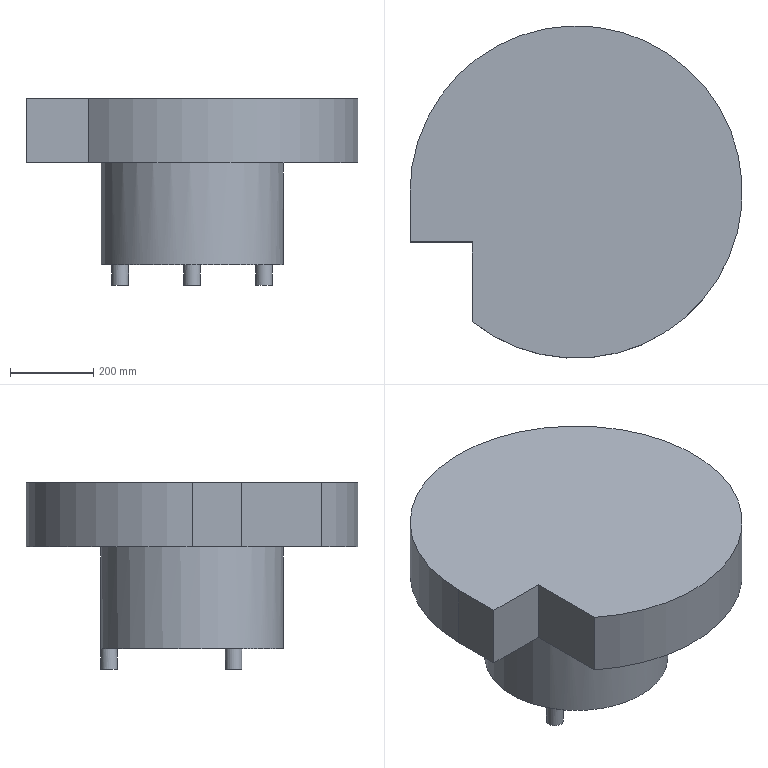Part | STEP file | ALIMENTADOR_ARRUELA | 1 solid | 14 faces | box 800 x 800 x 450 mm | volume 113086598 mm3 | plane 9 | cylinder 5 | commonest cylinder face diameters 40 x3 440 x1 800 x1
STEP:
#1=CARTESIAN_POINT('',(0.,0.,0.));
#2=DIRECTION('',(0.,0.,1.));
#3=DIRECTION('',(1.,0.,0.));
#4=AXIS2_PLACEMENT_3D('',#1,#2,#3);
#5=CARTESIAN_POINT('',(0.,220.,0.));
#6=VERTEX_POINT('',#5);
#7=CARTESIAN_POINT('',(-20.,200.,0.));
#8=VERTEX_POINT('',#7);
#9=CARTESIAN_POINT('',(0.,200.,0.));
#10=DIRECTION('',(0.,0.,-1.));
#11=DIRECTION('',(1.,0.,0.));
#12=AXIS2_PLACEMENT_3D('',#9,#10,#11);
#13=CIRCLE('',#12,20.);
#14=CARTESIAN_POINT('',(0.,200.,25.));
#15=DIRECTION('',(0.,0.,-1.));
#16=DIRECTION('',(1.,0.,0.));
#17=AXIS2_PLACEMENT_3D('',#14,#15,#16);
#18=CYLINDRICAL_SURFACE('',#17,20.);
#19=CARTESIAN_POINT('',(0.,25.));
#20=DIRECTION('',(1.,0.));
#21=VECTOR('',#20,1.);
#22=LINE('',#19,#21);
#23=(GEOMETRIC_REPRESENTATION_CONTEXT(2)PARAMETRIC_REPRESENTATION_CONTEXT()REPRESENTATION_CONTEXT('',''));
#24=DEFINITIONAL_REPRESENTATION('',(#22),#23);
#25=PCURVE('',#18,#24);
#26=CARTESIAN_POINT('',(0.,0.,0.));
#27=DIRECTION('',(0.,0.,-1.));
#28=DIRECTION('',(-1.,0.,0.));
#29=AXIS2_PLACEMENT_3D('',#26,#27,#28);
#30=PLANE('',#29);
#31=CARTESIAN_POINT('',(0.,200.));
#32=DIRECTION('',(-1.,0.));
#33=AXIS2_PLACEMENT_2D('',#31,#32);
#34=CIRCLE('',#33,20.);
#35=(GEOMETRIC_REPRESENTATION_CONTEXT(2)PARAMETRIC_REPRESENTATION_CONTEXT()REPRESENTATION_CONTEXT('',''));
#36=DEFINITIONAL_REPRESENTATION('',(#34),#35);
#37=PCURVE('',#30,#36);
#38=SURFACE_CURVE('',#13,(#25,#37),.PCURVE_S1.);
#39=EDGE_CURVE('',#6,#8,#38,.T.);
#40=ORIENTED_EDGE('',*,*,#39,.F.);
#41=CARTESIAN_POINT('',(0.,220.,50.));
#42=VERTEX_POINT('',#41);
#43=CARTESIAN_POINT('',(0.,220.,50.));
#44=CARTESIAN_POINT('',(0.,220.,0.));
#45=B_SPLINE_CURVE_WITH_KNOTS('',1,(#43,#44),.UNSPECIFIED.,.F.,.F.,(2,2),(-25.,25.),.PIECEWISE_BEZIER_KNOTS.);
#46=CARTESIAN_POINT('',(4.712,0.));
#47=DIRECTION('',(0.,1.));
#48=VECTOR('',#47,1.);
#49=LINE('',#46,#48);
#50=(GEOMETRIC_REPRESENTATION_CONTEXT(2)PARAMETRIC_REPRESENTATION_CONTEXT()REPRESENTATION_CONTEXT('',''));
#51=DEFINITIONAL_REPRESENTATION('',(#49),#50);
#52=PCURVE('',#18,#51);
#53=CARTESIAN_POINT('',(10.996,0.));
#54=DIRECTION('',(0.,1.));
#55=VECTOR('',#54,1.);
#56=LINE('',#53,#55);
#57=(GEOMETRIC_REPRESENTATION_CONTEXT(2)PARAMETRIC_REPRESENTATION_CONTEXT()REPRESENTATION_CONTEXT('',''));
#58=DEFINITIONAL_REPRESENTATION('',(#56),#57);
#59=PCURVE('',#18,#58);
#60=SEAM_CURVE('',#45,(#52,#59),.PCURVE_S1.);
#61=EDGE_CURVE('',#42,#6,#60,.T.);
#62=ORIENTED_EDGE('',*,*,#61,.F.);
#63=CARTESIAN_POINT('',(0.,220.,50.));
#64=VERTEX_POINT('',#63);
#65=CARTESIAN_POINT('',(0.,200.,50.));
#66=DIRECTION('',(0.,0.,-1.));
#67=DIRECTION('',(1.,0.,0.));
#68=AXIS2_PLACEMENT_3D('',#65,#66,#67);
#69=CIRCLE('',#68,20.);
#70=CARTESIAN_POINT('',(0.,-25.));
#71=DIRECTION('',(1.,0.));
#72=VECTOR('',#71,1.);
#73=LINE('',#70,#72);
#74=(GEOMETRIC_REPRESENTATION_CONTEXT(2)PARAMETRIC_REPRESENTATION_CONTEXT()REPRESENTATION_CONTEXT('',''));
#75=DEFINITIONAL_REPRESENTATION('',(#73),#74);
#76=PCURVE('',#18,#75);
#77=CARTESIAN_POINT('',(-220.,0.,50.));
#78=DIRECTION('',(0.,0.,1.));
#79=DIRECTION('',(1.,0.,0.));
#80=AXIS2_PLACEMENT_3D('',#77,#78,#79);
#81=PLANE('',#80);
#82=CARTESIAN_POINT('',(240.,200.));
#83=CARTESIAN_POINT('',(240.,165.359));
#84=CARTESIAN_POINT('',(210.,182.679));
#85=CARTESIAN_POINT('',(180.,200.));
#86=CARTESIAN_POINT('',(210.,217.321));
#87=CARTESIAN_POINT('',(240.,234.641));
#88=CARTESIAN_POINT('',(240.,200.));
#89=(BOUNDED_CURVE()B_SPLINE_CURVE(2,(#82,#83,#84,#85,#86,#87,#88),.UNSPECIFIED.,.T.,.F.)B_SPLINE_CURVE_WITH_KNOTS((1,2,2,2,2,1),(-2.094,0.,2.094,4.189,6.283,8.378),.UNSPECIFIED.)CURVE()GEOMETRIC_REPRESENTATION_ITEM()RATIONAL_B_SPLINE_CURVE((1.,0.5,1.,0.5,1.,0.5,1.))REPRESENTATION_ITEM(''));
#90=(GEOMETRIC_REPRESENTATION_CONTEXT(2)PARAMETRIC_REPRESENTATION_CONTEXT()REPRESENTATION_CONTEXT('',''));
#91=DEFINITIONAL_REPRESENTATION('',(#89),#90);
#92=PCURVE('',#81,#91);
#93=SURFACE_CURVE('',#69,(#76,#92),.PCURVE_S1.);
#94=EDGE_CURVE('',#64,#42,#93,.T.);
#95=ORIENTED_EDGE('',*,*,#94,.T.);
#96=ORIENTED_EDGE('',*,*,#61,.T.);
#97=CARTESIAN_POINT('',(0.,200.,0.));
#98=DIRECTION('',(0.,0.,-1.));
#99=DIRECTION('',(1.,0.,0.));
#100=AXIS2_PLACEMENT_3D('',#97,#98,#99);
#101=CIRCLE('',#100,20.);
#102=CARTESIAN_POINT('',(6.283,25.));
#103=DIRECTION('',(1.,0.));
#104=VECTOR('',#103,1.);
#105=LINE('',#102,#104);
#106=(GEOMETRIC_REPRESENTATION_CONTEXT(2)PARAMETRIC_REPRESENTATION_CONTEXT()REPRESENTATION_CONTEXT('',''));
#107=DEFINITIONAL_REPRESENTATION('',(#105),#106);
#108=PCURVE('',#18,#107);
#109=CARTESIAN_POINT('',(0.,200.));
#110=DIRECTION('',(-1.,0.));
#111=AXIS2_PLACEMENT_2D('',#109,#110);
#112=CIRCLE('',#111,20.);
#113=(GEOMETRIC_REPRESENTATION_CONTEXT(2)PARAMETRIC_REPRESENTATION_CONTEXT()REPRESENTATION_CONTEXT('',''));
#114=DEFINITIONAL_REPRESENTATION('',(#112),#113);
#115=PCURVE('',#30,#114);
#116=SURFACE_CURVE('',#101,(#108,#115),.PCURVE_S1.);
#117=EDGE_CURVE('',#8,#6,#116,.T.);
#118=ORIENTED_EDGE('',*,*,#117,.F.);
#119=EDGE_LOOP('',(#40,#62,#95,#96,#118));
#120=FACE_BOUND('',#119,.T.);
#121=ADVANCED_FACE('',(#120),#18,.T.);
#122=CARTESIAN_POINT('',(-190.526,-110.,50.));
#123=VERTEX_POINT('',#122);
#124=CARTESIAN_POINT('',(190.526,-110.,50.));
#125=VERTEX_POINT('',#124);
#126=CARTESIAN_POINT('',(0.,0.,50.));
#127=DIRECTION('',(0.,0.,1.));
#128=DIRECTION('',(1.,0.,0.));
#129=AXIS2_PLACEMENT_3D('',#126,#127,#128);
#130=CIRCLE('',#129,220.);
#131=CARTESIAN_POINT('',(220.,0.));
#132=DIRECTION('',(1.,0.));
#133=AXIS2_PLACEMENT_2D('',#131,#132);
#134=CIRCLE('',#133,220.);
#135=(GEOMETRIC_REPRESENTATION_CONTEXT(2)PARAMETRIC_REPRESENTATION_CONTEXT()REPRESENTATION_CONTEXT('',''));
#136=DEFINITIONAL_REPRESENTATION('',(#134),#135);
#137=PCURVE('',#81,#136);
#138=CARTESIAN_POINT('',(0.,0.,250.));
#139=DIRECTION('',(0.,0.,1.));
#140=DIRECTION('',(-0.8776,-0.4794,0.));
#141=AXIS2_PLACEMENT_3D('',#138,#139,#140);
#142=CYLINDRICAL_SURFACE('',#141,220.);
#143=CARTESIAN_POINT('',(-3.642,-200.));
#144=DIRECTION('',(1.,0.));
#145=VECTOR('',#144,1.);
#146=LINE('',#143,#145);
#147=(GEOMETRIC_REPRESENTATION_CONTEXT(2)PARAMETRIC_REPRESENTATION_CONTEXT()REPRESENTATION_CONTEXT('',''));
#148=DEFINITIONAL_REPRESENTATION('',(#146),#147);
#149=PCURVE('',#142,#148);
#150=SURFACE_CURVE('',#130,(#137,#149),.PCURVE_S1.);
#151=EDGE_CURVE('',#123,#125,#150,.T.);
#152=ORIENTED_EDGE('',*,*,#151,.T.);
#153=CARTESIAN_POINT('',(0.,0.,50.));
#154=DIRECTION('',(0.,0.,1.));
#155=DIRECTION('',(1.,0.,0.));
#156=AXIS2_PLACEMENT_3D('',#153,#154,#155);
#157=CIRCLE('',#156,220.);
#158=CARTESIAN_POINT('',(220.,0.));
#159=DIRECTION('',(1.,0.));
#160=AXIS2_PLACEMENT_2D('',#158,#159);
#161=CIRCLE('',#160,220.);
#162=(GEOMETRIC_REPRESENTATION_CONTEXT(2)PARAMETRIC_REPRESENTATION_CONTEXT()REPRESENTATION_CONTEXT('',''));
#163=DEFINITIONAL_REPRESENTATION('',(#161),#162);
#164=PCURVE('',#81,#163);
#165=CARTESIAN_POINT('',(-3.642,-200.));
#166=DIRECTION('',(1.,0.));
#167=VECTOR('',#166,1.);
#168=LINE('',#165,#167);
#169=(GEOMETRIC_REPRESENTATION_CONTEXT(2)PARAMETRIC_REPRESENTATION_CONTEXT()REPRESENTATION_CONTEXT('',''));
#170=DEFINITIONAL_REPRESENTATION('',(#168),#169);
#171=PCURVE('',#142,#170);
#172=SURFACE_CURVE('',#157,(#164,#171),.PCURVE_S1.);
#173=EDGE_CURVE('',#125,#42,#172,.T.);
#174=ORIENTED_EDGE('',*,*,#173,.T.);
#175=CARTESIAN_POINT('',(-193.068,-105.474,50.));
#176=VERTEX_POINT('',#175);
#177=CARTESIAN_POINT('',(0.,0.,50.));
#178=DIRECTION('',(0.,0.,1.));
#179=DIRECTION('',(1.,0.,0.));
#180=AXIS2_PLACEMENT_3D('',#177,#178,#179);
#181=CIRCLE('',#180,220.);
#182=CARTESIAN_POINT('',(220.,0.));
#183=DIRECTION('',(1.,0.));
#184=AXIS2_PLACEMENT_2D('',#182,#183);
#185=CIRCLE('',#184,220.);
#186=(GEOMETRIC_REPRESENTATION_CONTEXT(2)PARAMETRIC_REPRESENTATION_CONTEXT()REPRESENTATION_CONTEXT('',''));
#187=DEFINITIONAL_REPRESENTATION('',(#185),#186);
#188=PCURVE('',#81,#187);
#189=CARTESIAN_POINT('',(2.642,-200.));
#190=DIRECTION('',(1.,0.));
#191=VECTOR('',#190,1.);
#192=LINE('',#189,#191);
#193=(GEOMETRIC_REPRESENTATION_CONTEXT(2)PARAMETRIC_REPRESENTATION_CONTEXT()REPRESENTATION_CONTEXT('',''));
#194=DEFINITIONAL_REPRESENTATION('',(#192),#193);
#195=PCURVE('',#142,#194);
#196=SURFACE_CURVE('',#181,(#188,#195),.PCURVE_S1.);
#197=EDGE_CURVE('',#42,#176,#196,.T.);
#198=ORIENTED_EDGE('',*,*,#197,.T.);
#199=CARTESIAN_POINT('',(0.,0.,50.));
#200=DIRECTION('',(0.,0.,1.));
#201=DIRECTION('',(1.,0.,0.));
#202=AXIS2_PLACEMENT_3D('',#199,#200,#201);
#203=CIRCLE('',#202,220.);
#204=CARTESIAN_POINT('',(220.,0.));
#205=DIRECTION('',(1.,0.));
#206=AXIS2_PLACEMENT_2D('',#204,#205);
#207=CIRCLE('',#206,220.);
#208=(GEOMETRIC_REPRESENTATION_CONTEXT(2)PARAMETRIC_REPRESENTATION_CONTEXT()REPRESENTATION_CONTEXT('',''));
#209=DEFINITIONAL_REPRESENTATION('',(#207),#208);
#210=PCURVE('',#81,#209);
#211=CARTESIAN_POINT('',(-3.642,-200.));
#212=DIRECTION('',(1.,0.));
#213=VECTOR('',#212,1.);
#214=LINE('',#211,#213);
#215=(GEOMETRIC_REPRESENTATION_CONTEXT(2)PARAMETRIC_REPRESENTATION_CONTEXT()REPRESENTATION_CONTEXT('',''));
#216=DEFINITIONAL_REPRESENTATION('',(#214),#215);
#217=PCURVE('',#142,#216);
#218=SURFACE_CURVE('',#203,(#210,#217),.PCURVE_S1.);
#219=EDGE_CURVE('',#176,#123,#218,.T.);
#220=ORIENTED_EDGE('',*,*,#219,.T.);
#221=EDGE_LOOP('',(#152,#174,#198,#220));
#222=FACE_BOUND('',#221,.F.);
#223=CARTESIAN_POINT('',(190.526,-110.,50.));
#224=VERTEX_POINT('',#223);
#225=CARTESIAN_POINT('',(173.205,-100.,50.));
#226=DIRECTION('',(0.,0.,1.));
#227=DIRECTION('',(1.,0.,0.));
#228=AXIS2_PLACEMENT_3D('',#225,#226,#227);
#229=CIRCLE('',#228,20.);
#230=CARTESIAN_POINT('',(393.205,-100.));
#231=DIRECTION('',(1.,0.));
#232=AXIS2_PLACEMENT_2D('',#230,#231);
#233=CIRCLE('',#232,20.);
#234=(GEOMETRIC_REPRESENTATION_CONTEXT(2)PARAMETRIC_REPRESENTATION_CONTEXT()REPRESENTATION_CONTEXT('',''));
#235=DEFINITIONAL_REPRESENTATION('',(#233),#234);
#236=PCURVE('',#81,#235);
#237=CARTESIAN_POINT('',(173.205,-100.,25.));
#238=DIRECTION('',(0.,0.,-1.));
#239=DIRECTION('',(-0.5,-0.866,0.));
#240=AXIS2_PLACEMENT_3D('',#237,#238,#239);
#241=CYLINDRICAL_SURFACE('',#240,20.);
#242=CARTESIAN_POINT('',(16.755,-25.));
#243=DIRECTION('',(-1.,0.));
#244=VECTOR('',#243,1.);
#245=LINE('',#242,#244);
#246=(GEOMETRIC_REPRESENTATION_CONTEXT(2)PARAMETRIC_REPRESENTATION_CONTEXT()REPRESENTATION_CONTEXT('',''));
#247=DEFINITIONAL_REPRESENTATION('',(#245),#246);
#248=PCURVE('',#241,#247);
#249=SURFACE_CURVE('',#229,(#236,#248),.PCURVE_S1.);
#250=EDGE_CURVE('',#125,#224,#249,.T.);
#251=ORIENTED_EDGE('',*,*,#250,.F.);
#252=EDGE_LOOP('',(#251));
#253=FACE_BOUND('',#252,.F.);
#254=ORIENTED_EDGE('',*,*,#94,.T.);
#255=EDGE_LOOP('',(#254));
#256=FACE_BOUND('',#255,.F.);
#257=CARTESIAN_POINT('',(-190.526,-110.,50.));
#258=VERTEX_POINT('',#257);
#259=CARTESIAN_POINT('',(-173.205,-100.,50.));
#260=DIRECTION('',(0.,0.,1.));
#261=DIRECTION('',(1.,0.,0.));
#262=AXIS2_PLACEMENT_3D('',#259,#260,#261);
#263=CIRCLE('',#262,20.);
#264=CARTESIAN_POINT('',(46.795,-100.));
#265=DIRECTION('',(1.,0.));
#266=AXIS2_PLACEMENT_2D('',#264,#265);
#267=CIRCLE('',#266,20.);
#268=(GEOMETRIC_REPRESENTATION_CONTEXT(2)PARAMETRIC_REPRESENTATION_CONTEXT()REPRESENTATION_CONTEXT('',''));
#269=DEFINITIONAL_REPRESENTATION('',(#267),#268);
#270=PCURVE('',#81,#269);
#271=CARTESIAN_POINT('',(-173.205,-100.,25.));
#272=DIRECTION('',(0.,0.,-1.));
#273=DIRECTION('',(-0.5,0.866,0.));
#274=AXIS2_PLACEMENT_3D('',#271,#272,#273);
#275=CYLINDRICAL_SURFACE('',#274,20.);
#276=CARTESIAN_POINT('',(14.661,-25.));
#277=DIRECTION('',(-1.,0.));
#278=VECTOR('',#277,1.);
#279=LINE('',#276,#278);
#280=(GEOMETRIC_REPRESENTATION_CONTEXT(2)PARAMETRIC_REPRESENTATION_CONTEXT()REPRESENTATION_CONTEXT('',''));
#281=DEFINITIONAL_REPRESENTATION('',(#279),#280);
#282=PCURVE('',#275,#281);
#283=SURFACE_CURVE('',#263,(#270,#282),.PCURVE_S1.);
#284=EDGE_CURVE('',#258,#123,#283,.T.);
#285=ORIENTED_EDGE('',*,*,#284,.F.);
#286=EDGE_LOOP('',(#285));
#287=FACE_BOUND('',#286,.F.);
#288=ADVANCED_FACE('',(#222,#253,#256,#287),#81,.F.);
#289=ORIENTED_EDGE('',*,*,#117,.T.);
#290=ORIENTED_EDGE('',*,*,#39,.T.);
#291=EDGE_LOOP('',(#289,#290));
#292=FACE_BOUND('',#291,.T.);
#293=ADVANCED_FACE('',(#292),#30,.T.);
#294=ORIENTED_EDGE('',*,*,#197,.T.);
#295=CARTESIAN_POINT('',(-193.068,-105.474,295.));
#296=VERTEX_POINT('',#295);
#297=CARTESIAN_POINT('',(-193.068,-105.474,50.));
#298=CARTESIAN_POINT('',(-193.068,-105.474,295.));
#299=B_SPLINE_CURVE_WITH_KNOTS('',1,(#297,#298),.UNSPECIFIED.,.F.,.F.,(2,2),(-200.,45.),.PIECEWISE_BEZIER_KNOTS.);
#300=CARTESIAN_POINT('',(6.283,0.));
#301=DIRECTION('',(0.,1.));
#302=VECTOR('',#301,1.);
#303=LINE('',#300,#302);
#304=(GEOMETRIC_REPRESENTATION_CONTEXT(2)PARAMETRIC_REPRESENTATION_CONTEXT()REPRESENTATION_CONTEXT('',''));
#305=DEFINITIONAL_REPRESENTATION('',(#303),#304);
#306=PCURVE('',#142,#305);
#307=CARTESIAN_POINT('',(0.,0.));
#308=DIRECTION('',(0.,1.));
#309=VECTOR('',#308,1.);
#310=LINE('',#307,#309);
#311=(GEOMETRIC_REPRESENTATION_CONTEXT(2)PARAMETRIC_REPRESENTATION_CONTEXT()REPRESENTATION_CONTEXT('',''));
#312=DEFINITIONAL_REPRESENTATION('',(#310),#311);
#313=PCURVE('',#142,#312);
#314=SEAM_CURVE('',#299,(#306,#313),.PCURVE_S1.);
#315=EDGE_CURVE('',#176,#296,#314,.T.);
#316=ORIENTED_EDGE('',*,*,#315,.T.);
#317=CARTESIAN_POINT('',(0.,0.,295.));
#318=DIRECTION('',(0.,0.,1.));
#319=DIRECTION('',(1.,0.,0.));
#320=AXIS2_PLACEMENT_3D('',#317,#318,#319);
#321=CIRCLE('',#320,220.);
#322=CARTESIAN_POINT('',(-3.642,45.));
#323=DIRECTION('',(1.,0.));
#324=VECTOR('',#323,1.);
#325=LINE('',#322,#324);
#326=(GEOMETRIC_REPRESENTATION_CONTEXT(2)PARAMETRIC_REPRESENTATION_CONTEXT()REPRESENTATION_CONTEXT('',''));
#327=DEFINITIONAL_REPRESENTATION('',(#325),#326);
#328=PCURVE('',#142,#327);
#329=CARTESIAN_POINT('',(-220.,0.,295.));
#330=DIRECTION('',(0.,0.,1.));
#331=DIRECTION('',(1.,0.,0.));
#332=AXIS2_PLACEMENT_3D('',#329,#330,#331);
#333=PLANE('',#332);
#334=CARTESIAN_POINT('',(220.,0.));
#335=DIRECTION('',(1.,0.));
#336=AXIS2_PLACEMENT_2D('',#334,#335);
#337=CIRCLE('',#336,220.);
#338=(GEOMETRIC_REPRESENTATION_CONTEXT(2)PARAMETRIC_REPRESENTATION_CONTEXT()REPRESENTATION_CONTEXT('',''));
#339=DEFINITIONAL_REPRESENTATION('',(#337),#338);
#340=PCURVE('',#333,#339);
#341=SURFACE_CURVE('',#321,(#328,#340),.PCURVE_S1.);
#342=EDGE_CURVE('',#296,#296,#341,.T.);
#343=ORIENTED_EDGE('',*,*,#342,.F.);
#344=ORIENTED_EDGE('',*,*,#315,.F.);
#345=ORIENTED_EDGE('',*,*,#219,.T.);
#346=ORIENTED_EDGE('',*,*,#151,.T.);
#347=ORIENTED_EDGE('',*,*,#173,.T.);
#348=EDGE_LOOP('',(#294,#316,#343,#344,#345,#346,#347));
#349=FACE_BOUND('',#348,.T.);
#350=ADVANCED_FACE('',(#349),#142,.T.);
#351=CARTESIAN_POINT('',(-250.,-120.,295.));
#352=VERTEX_POINT('',#351);
#353=CARTESIAN_POINT('',(-250.,-312.25,295.));
#354=VERTEX_POINT('',#353);
#355=CARTESIAN_POINT('',(-250.,-120.,295.));
#356=DIRECTION('',(0.,-1.,0.));
#357=VECTOR('',#356,1.);
#358=LINE('',#355,#357);
#359=CARTESIAN_POINT('',(-30.,-120.));
#360=DIRECTION('',(0.,-1.));
#361=VECTOR('',#360,1.);
#362=LINE('',#359,#361);
#363=(GEOMETRIC_REPRESENTATION_CONTEXT(2)PARAMETRIC_REPRESENTATION_CONTEXT()REPRESENTATION_CONTEXT('',''));
#364=DEFINITIONAL_REPRESENTATION('',(#362),#363);
#365=PCURVE('',#333,#364);
#366=CARTESIAN_POINT('',(-250.,-120.,450.));
#367=DIRECTION('',(1.,0.,0.));
#368=DIRECTION('',(0.,0.,-1.));
#369=AXIS2_PLACEMENT_3D('',#366,#367,#368);
#370=PLANE('',#369);
#371=CARTESIAN_POINT('',(155.,0.));
#372=DIRECTION('',(0.,-1.));
#373=VECTOR('',#372,1.);
#374=LINE('',#371,#373);
#375=(GEOMETRIC_REPRESENTATION_CONTEXT(2)PARAMETRIC_REPRESENTATION_CONTEXT()REPRESENTATION_CONTEXT('',''));
#376=DEFINITIONAL_REPRESENTATION('',(#374),#375);
#377=PCURVE('',#370,#376);
#378=SURFACE_CURVE('',#358,(#365,#377),.PCURVE_S1.);
#379=EDGE_CURVE('',#352,#354,#378,.T.);
#380=ORIENTED_EDGE('',*,*,#379,.F.);
#381=CARTESIAN_POINT('',(-400.,-120.,295.));
#382=VERTEX_POINT('',#381);
#383=CARTESIAN_POINT('',(-250.,-120.,295.));
#384=DIRECTION('',(-1.,0.,0.));
#385=VECTOR('',#384,1.);
#386=LINE('',#383,#385);
#387=CARTESIAN_POINT('',(-30.,-120.));
#388=DIRECTION('',(-1.,0.));
#389=VECTOR('',#388,1.);
#390=LINE('',#387,#389);
#391=(GEOMETRIC_REPRESENTATION_CONTEXT(2)PARAMETRIC_REPRESENTATION_CONTEXT()REPRESENTATION_CONTEXT('',''));
#392=DEFINITIONAL_REPRESENTATION('',(#390),#391);
#393=PCURVE('',#333,#392);
#394=CARTESIAN_POINT('',(-250.,-120.,450.));
#395=DIRECTION('',(0.,-1.,0.));
#396=DIRECTION('',(0.,0.,-1.));
#397=AXIS2_PLACEMENT_3D('',#394,#395,#396);
#398=PLANE('',#397);
#399=CARTESIAN_POINT('',(155.,0.));
#400=DIRECTION('',(0.,-1.));
#401=VECTOR('',#400,1.);
#402=LINE('',#399,#401);
#403=(GEOMETRIC_REPRESENTATION_CONTEXT(2)PARAMETRIC_REPRESENTATION_CONTEXT()REPRESENTATION_CONTEXT('',''));
#404=DEFINITIONAL_REPRESENTATION('',(#402),#403);
#405=PCURVE('',#398,#404);
#406=SURFACE_CURVE('',#386,(#393,#405),.PCURVE_S1.);
#407=EDGE_CURVE('',#352,#382,#406,.T.);
#408=ORIENTED_EDGE('',*,*,#407,.T.);
#409=CARTESIAN_POINT('',(-400.,0.,295.));
#410=VERTEX_POINT('',#409);
#411=CARTESIAN_POINT('',(-400.,0.,295.));
#412=DIRECTION('',(0.,-1.,0.));
#413=VECTOR('',#412,1.);
#414=LINE('',#411,#413);
#415=CARTESIAN_POINT('',(-180.,0.));
#416=DIRECTION('',(0.,-1.));
#417=VECTOR('',#416,1.);
#418=LINE('',#415,#417);
#419=(GEOMETRIC_REPRESENTATION_CONTEXT(2)PARAMETRIC_REPRESENTATION_CONTEXT()REPRESENTATION_CONTEXT('',''));
#420=DEFINITIONAL_REPRESENTATION('',(#418),#419);
#421=PCURVE('',#333,#420);
#422=CARTESIAN_POINT('',(-400.,0.,450.));
#423=DIRECTION('',(1.,0.,0.));
#424=DIRECTION('',(0.,0.,-1.));
#425=AXIS2_PLACEMENT_3D('',#422,#423,#424);
#426=PLANE('',#425);
#427=CARTESIAN_POINT('',(155.,0.));
#428=DIRECTION('',(0.,-1.));
#429=VECTOR('',#428,1.);
#430=LINE('',#427,#429);
#431=(GEOMETRIC_REPRESENTATION_CONTEXT(2)PARAMETRIC_REPRESENTATION_CONTEXT()REPRESENTATION_CONTEXT('',''));
#432=DEFINITIONAL_REPRESENTATION('',(#430),#431);
#433=PCURVE('',#426,#432);
#434=SURFACE_CURVE('',#414,(#421,#433),.PCURVE_S1.);
#435=EDGE_CURVE('',#410,#382,#434,.T.);
#436=ORIENTED_EDGE('',*,*,#435,.F.);
#437=CARTESIAN_POINT('',(0.,0.,295.));
#438=DIRECTION('',(0.,0.,1.));
#439=DIRECTION('',(1.,0.,0.));
#440=AXIS2_PLACEMENT_3D('',#437,#438,#439);
#441=CIRCLE('',#440,400.);
#442=CARTESIAN_POINT('',(220.,0.));
#443=DIRECTION('',(1.,0.));
#444=AXIS2_PLACEMENT_2D('',#442,#443);
#445=CIRCLE('',#444,400.);
#446=(GEOMETRIC_REPRESENTATION_CONTEXT(2)PARAMETRIC_REPRESENTATION_CONTEXT()REPRESENTATION_CONTEXT('',''));
#447=DEFINITIONAL_REPRESENTATION('',(#445),#446);
#448=PCURVE('',#333,#447);
#449=CARTESIAN_POINT('',(0.,0.,250.));
#450=DIRECTION('',(0.,0.,1.));
#451=DIRECTION('',(-0.8776,-0.4794,0.));
#452=AXIS2_PLACEMENT_3D('',#449,#450,#451);
#453=CYLINDRICAL_SURFACE('',#452,400.);
#454=CARTESIAN_POINT('',(-3.642,45.));
#455=DIRECTION('',(1.,0.));
#456=VECTOR('',#455,1.);
#457=LINE('',#454,#456);
#458=(GEOMETRIC_REPRESENTATION_CONTEXT(2)PARAMETRIC_REPRESENTATION_CONTEXT()REPRESENTATION_CONTEXT('',''));
#459=DEFINITIONAL_REPRESENTATION('',(#457),#458);
#460=PCURVE('',#453,#459);
#461=SURFACE_CURVE('',#441,(#448,#460),.PCURVE_S1.);
#462=EDGE_CURVE('',#354,#410,#461,.T.);
#463=ORIENTED_EDGE('',*,*,#462,.F.);
#464=EDGE_LOOP('',(#380,#408,#436,#463));
#465=FACE_BOUND('',#464,.T.);
#466=ORIENTED_EDGE('',*,*,#342,.T.);
#467=EDGE_LOOP('',(#466));
#468=FACE_BOUND('',#467,.T.);
#469=ADVANCED_FACE('',(#465,#468),#333,.F.);
#470=ORIENTED_EDGE('',*,*,#462,.T.);
#471=CARTESIAN_POINT('',(-400.,0.,450.));
#472=VERTEX_POINT('',#471);
#473=CARTESIAN_POINT('',(-400.,0.,295.));
#474=DIRECTION('',(0.,0.,1.));
#475=VECTOR('',#474,1.);
#476=LINE('',#473,#475);
#477=CARTESIAN_POINT('',(5.783,45.));
#478=DIRECTION('',(0.,1.));
#479=VECTOR('',#478,1.);
#480=LINE('',#477,#479);
#481=(GEOMETRIC_REPRESENTATION_CONTEXT(2)PARAMETRIC_REPRESENTATION_CONTEXT()REPRESENTATION_CONTEXT('',''));
#482=DEFINITIONAL_REPRESENTATION('',(#480),#481);
#483=PCURVE('',#453,#482);
#484=CARTESIAN_POINT('',(155.,0.));
#485=DIRECTION('',(-1.,0.));
#486=VECTOR('',#485,1.);
#487=LINE('',#484,#486);
#488=(GEOMETRIC_REPRESENTATION_CONTEXT(2)PARAMETRIC_REPRESENTATION_CONTEXT()REPRESENTATION_CONTEXT('',''));
#489=DEFINITIONAL_REPRESENTATION('',(#487),#488);
#490=PCURVE('',#426,#489);
#491=SURFACE_CURVE('',#476,(#483,#490),.PCURVE_S1.);
#492=EDGE_CURVE('',#410,#472,#491,.T.);
#493=ORIENTED_EDGE('',*,*,#492,.T.);
#494=CARTESIAN_POINT('',(-250.,-312.25,450.));
#495=VERTEX_POINT('',#494);
#496=CARTESIAN_POINT('',(0.,0.,450.));
#497=DIRECTION('',(0.,0.,1.));
#498=DIRECTION('',(1.,0.,0.));
#499=AXIS2_PLACEMENT_3D('',#496,#497,#498);
#500=CIRCLE('',#499,400.);
#501=CARTESIAN_POINT('',(-3.642,200.));
#502=DIRECTION('',(1.,0.));
#503=VECTOR('',#502,1.);
#504=LINE('',#501,#503);
#505=(GEOMETRIC_REPRESENTATION_CONTEXT(2)PARAMETRIC_REPRESENTATION_CONTEXT()REPRESENTATION_CONTEXT('',''));
#506=DEFINITIONAL_REPRESENTATION('',(#504),#505);
#507=PCURVE('',#453,#506);
#508=CARTESIAN_POINT('',(-400.,0.,450.));
#509=DIRECTION('',(0.,0.,1.));
#510=DIRECTION('',(1.,0.,0.));
#511=AXIS2_PLACEMENT_3D('',#508,#509,#510);
#512=PLANE('',#511);
#513=CARTESIAN_POINT('',(400.,0.));
#514=DIRECTION('',(1.,0.));
#515=AXIS2_PLACEMENT_2D('',#513,#514);
#516=CIRCLE('',#515,400.);
#517=(GEOMETRIC_REPRESENTATION_CONTEXT(2)PARAMETRIC_REPRESENTATION_CONTEXT()REPRESENTATION_CONTEXT('',''));
#518=DEFINITIONAL_REPRESENTATION('',(#516),#517);
#519=PCURVE('',#512,#518);
#520=SURFACE_CURVE('',#500,(#507,#519),.PCURVE_S1.);
#521=EDGE_CURVE('',#495,#472,#520,.T.);
#522=ORIENTED_EDGE('',*,*,#521,.F.);
#523=CARTESIAN_POINT('',(-250.,-312.25,295.));
#524=DIRECTION('',(0.,0.,1.));
#525=VECTOR('',#524,1.);
#526=LINE('',#523,#525);
#527=CARTESIAN_POINT('',(0.3957,45.));
#528=DIRECTION('',(0.,1.));
#529=VECTOR('',#528,1.);
#530=LINE('',#527,#529);
#531=(GEOMETRIC_REPRESENTATION_CONTEXT(2)PARAMETRIC_REPRESENTATION_CONTEXT()REPRESENTATION_CONTEXT('',''));
#532=DEFINITIONAL_REPRESENTATION('',(#530),#531);
#533=PCURVE('',#453,#532);
#534=CARTESIAN_POINT('',(155.,-192.25));
#535=DIRECTION('',(-1.,0.));
#536=VECTOR('',#535,1.);
#537=LINE('',#534,#536);
#538=(GEOMETRIC_REPRESENTATION_CONTEXT(2)PARAMETRIC_REPRESENTATION_CONTEXT()REPRESENTATION_CONTEXT('',''));
#539=DEFINITIONAL_REPRESENTATION('',(#537),#538);
#540=PCURVE('',#370,#539);
#541=SURFACE_CURVE('',#526,(#533,#540),.PCURVE_S1.);
#542=EDGE_CURVE('',#354,#495,#541,.T.);
#543=ORIENTED_EDGE('',*,*,#542,.F.);
#544=EDGE_LOOP('',(#470,#493,#522,#543));
#545=FACE_BOUND('',#544,.T.);
#546=ADVANCED_FACE('',(#545),#453,.T.);
#547=ORIENTED_EDGE('',*,*,#435,.T.);
#548=CARTESIAN_POINT('',(-400.,-120.,450.));
#549=VERTEX_POINT('',#548);
#550=CARTESIAN_POINT('',(-400.,-120.,450.));
#551=DIRECTION('',(0.,0.,-1.));
#552=VECTOR('',#551,1.);
#553=LINE('',#550,#552);
#554=CARTESIAN_POINT('',(0.,-120.));
#555=DIRECTION('',(1.,0.));
#556=VECTOR('',#555,1.);
#557=LINE('',#554,#556);
#558=(GEOMETRIC_REPRESENTATION_CONTEXT(2)PARAMETRIC_REPRESENTATION_CONTEXT()REPRESENTATION_CONTEXT('',''));
#559=DEFINITIONAL_REPRESENTATION('',(#557),#558);
#560=PCURVE('',#426,#559);
#561=CARTESIAN_POINT('',(0.,-150.));
#562=DIRECTION('',(1.,0.));
#563=VECTOR('',#562,1.);
#564=LINE('',#561,#563);
#565=(GEOMETRIC_REPRESENTATION_CONTEXT(2)PARAMETRIC_REPRESENTATION_CONTEXT()REPRESENTATION_CONTEXT('',''));
#566=DEFINITIONAL_REPRESENTATION('',(#564),#565);
#567=PCURVE('',#398,#566);
#568=SURFACE_CURVE('',#553,(#560,#567),.PCURVE_S1.);
#569=EDGE_CURVE('',#549,#382,#568,.T.);
#570=ORIENTED_EDGE('',*,*,#569,.F.);
#571=CARTESIAN_POINT('',(-400.,0.,450.));
#572=DIRECTION('',(0.,-1.,0.));
#573=VECTOR('',#572,1.);
#574=LINE('',#571,#573);
#575=CARTESIAN_POINT('',(0.,0.));
#576=DIRECTION('',(0.,-1.));
#577=VECTOR('',#576,1.);
#578=LINE('',#575,#577);
#579=(GEOMETRIC_REPRESENTATION_CONTEXT(2)PARAMETRIC_REPRESENTATION_CONTEXT()REPRESENTATION_CONTEXT('',''));
#580=DEFINITIONAL_REPRESENTATION('',(#578),#579);
#581=PCURVE('',#426,#580);
#582=CARTESIAN_POINT('',(0.,0.));
#583=DIRECTION('',(0.,-1.));
#584=VECTOR('',#583,1.);
#585=LINE('',#582,#584);
#586=(GEOMETRIC_REPRESENTATION_CONTEXT(2)PARAMETRIC_REPRESENTATION_CONTEXT()REPRESENTATION_CONTEXT('',''));
#587=DEFINITIONAL_REPRESENTATION('',(#585),#586);
#588=PCURVE('',#512,#587);
#589=SURFACE_CURVE('',#574,(#581,#588),.PCURVE_S1.);
#590=EDGE_CURVE('',#472,#549,#589,.T.);
#591=ORIENTED_EDGE('',*,*,#590,.F.);
#592=ORIENTED_EDGE('',*,*,#492,.F.);
#593=EDGE_LOOP('',(#547,#570,#591,#592));
#594=FACE_BOUND('',#593,.T.);
#595=ADVANCED_FACE('',(#594),#426,.F.);
#596=CARTESIAN_POINT('',(-250.,-120.,450.));
#597=VERTEX_POINT('',#596);
#598=CARTESIAN_POINT('',(-250.,-120.,450.));
#599=DIRECTION('',(0.,0.,-1.));
#600=VECTOR('',#599,1.);
#601=LINE('',#598,#600);
#602=CARTESIAN_POINT('',(0.,0.));
#603=DIRECTION('',(1.,0.));
#604=VECTOR('',#603,1.);
#605=LINE('',#602,#604);
#606=(GEOMETRIC_REPRESENTATION_CONTEXT(2)PARAMETRIC_REPRESENTATION_CONTEXT()REPRESENTATION_CONTEXT('',''));
#607=DEFINITIONAL_REPRESENTATION('',(#605),#606);
#608=PCURVE('',#398,#607);
#609=CARTESIAN_POINT('',(0.,0.));
#610=DIRECTION('',(1.,0.));
#611=VECTOR('',#610,1.);
#612=LINE('',#609,#611);
#613=(GEOMETRIC_REPRESENTATION_CONTEXT(2)PARAMETRIC_REPRESENTATION_CONTEXT()REPRESENTATION_CONTEXT('',''));
#614=DEFINITIONAL_REPRESENTATION('',(#612),#613);
#615=PCURVE('',#370,#614);
#616=SURFACE_CURVE('',#601,(#608,#615),.PCURVE_S1.);
#617=EDGE_CURVE('',#597,#352,#616,.T.);
#618=ORIENTED_EDGE('',*,*,#617,.F.);
#619=CARTESIAN_POINT('',(-400.,-120.,450.));
#620=DIRECTION('',(1.,0.,0.));
#621=VECTOR('',#620,1.);
#622=LINE('',#619,#621);
#623=CARTESIAN_POINT('',(0.,-150.));
#624=DIRECTION('',(0.,1.));
#625=VECTOR('',#624,1.);
#626=LINE('',#623,#625);
#627=(GEOMETRIC_REPRESENTATION_CONTEXT(2)PARAMETRIC_REPRESENTATION_CONTEXT()REPRESENTATION_CONTEXT('',''));
#628=DEFINITIONAL_REPRESENTATION('',(#626),#627);
#629=PCURVE('',#398,#628);
#630=CARTESIAN_POINT('',(0.,-120.));
#631=DIRECTION('',(1.,0.));
#632=VECTOR('',#631,1.);
#633=LINE('',#630,#632);
#634=(GEOMETRIC_REPRESENTATION_CONTEXT(2)PARAMETRIC_REPRESENTATION_CONTEXT()REPRESENTATION_CONTEXT('',''));
#635=DEFINITIONAL_REPRESENTATION('',(#633),#634);
#636=PCURVE('',#512,#635);
#637=SURFACE_CURVE('',#622,(#629,#636),.PCURVE_S1.);
#638=EDGE_CURVE('',#549,#597,#637,.T.);
#639=ORIENTED_EDGE('',*,*,#638,.F.);
#640=ORIENTED_EDGE('',*,*,#569,.T.);
#641=ORIENTED_EDGE('',*,*,#407,.F.);
#642=EDGE_LOOP('',(#618,#639,#640,#641));
#643=FACE_BOUND('',#642,.T.);
#644=ADVANCED_FACE('',(#643),#398,.T.);
#645=ORIENTED_EDGE('',*,*,#379,.T.);
#646=ORIENTED_EDGE('',*,*,#542,.T.);
#647=CARTESIAN_POINT('',(-250.,-120.,450.));
#648=DIRECTION('',(0.,-1.,0.));
#649=VECTOR('',#648,1.);
#650=LINE('',#647,#649);
#651=CARTESIAN_POINT('',(0.,0.));
#652=DIRECTION('',(0.,-1.));
#653=VECTOR('',#652,1.);
#654=LINE('',#651,#653);
#655=(GEOMETRIC_REPRESENTATION_CONTEXT(2)PARAMETRIC_REPRESENTATION_CONTEXT()REPRESENTATION_CONTEXT('',''));
#656=DEFINITIONAL_REPRESENTATION('',(#654),#655);
#657=PCURVE('',#370,#656);
#658=CARTESIAN_POINT('',(150.,-120.));
#659=DIRECTION('',(0.,-1.));
#660=VECTOR('',#659,1.);
#661=LINE('',#658,#660);
#662=(GEOMETRIC_REPRESENTATION_CONTEXT(2)PARAMETRIC_REPRESENTATION_CONTEXT()REPRESENTATION_CONTEXT('',''));
#663=DEFINITIONAL_REPRESENTATION('',(#661),#662);
#664=PCURVE('',#512,#663);
#665=SURFACE_CURVE('',#650,(#657,#664),.PCURVE_S1.);
#666=EDGE_CURVE('',#597,#495,#665,.T.);
#667=ORIENTED_EDGE('',*,*,#666,.F.);
#668=ORIENTED_EDGE('',*,*,#617,.T.);
#669=EDGE_LOOP('',(#645,#646,#667,#668));
#670=FACE_BOUND('',#669,.T.);
#671=ADVANCED_FACE('',(#670),#370,.F.);
#672=ORIENTED_EDGE('',*,*,#521,.T.);
#673=ORIENTED_EDGE('',*,*,#590,.T.);
#674=ORIENTED_EDGE('',*,*,#638,.T.);
#675=ORIENTED_EDGE('',*,*,#666,.T.);
#676=EDGE_LOOP('',(#672,#673,#674,#675));
#677=FACE_BOUND('',#676,.T.);
#678=ADVANCED_FACE('',(#677),#512,.T.);
#679=CARTESIAN_POINT('',(190.526,-110.,0.));
#680=VERTEX_POINT('',#679);
#681=CARTESIAN_POINT('',(183.205,-82.679,0.));
#682=VERTEX_POINT('',#681);
#683=CARTESIAN_POINT('',(173.205,-100.,0.));
#684=DIRECTION('',(0.,0.,-1.));
#685=DIRECTION('',(1.,0.,0.));
#686=AXIS2_PLACEMENT_3D('',#683,#684,#685);
#687=CIRCLE('',#686,20.);
#688=CARTESIAN_POINT('',(4.189,25.));
#689=DIRECTION('',(1.,0.));
#690=VECTOR('',#689,1.);
#691=LINE('',#688,#690);
#692=(GEOMETRIC_REPRESENTATION_CONTEXT(2)PARAMETRIC_REPRESENTATION_CONTEXT()REPRESENTATION_CONTEXT('',''));
#693=DEFINITIONAL_REPRESENTATION('',(#691),#692);
#694=PCURVE('',#241,#693);
#695=CARTESIAN_POINT('',(0.,0.,0.));
#696=DIRECTION('',(0.,0.,-1.));
#697=DIRECTION('',(-1.,0.,0.));
#698=AXIS2_PLACEMENT_3D('',#695,#696,#697);
#699=PLANE('',#698);
#700=CARTESIAN_POINT('',(-173.205,-100.));
#701=DIRECTION('',(-1.,0.));
#702=AXIS2_PLACEMENT_2D('',#700,#701);
#703=CIRCLE('',#702,20.);
#704=(GEOMETRIC_REPRESENTATION_CONTEXT(2)PARAMETRIC_REPRESENTATION_CONTEXT()REPRESENTATION_CONTEXT('',''));
#705=DEFINITIONAL_REPRESENTATION('',(#703),#704);
#706=PCURVE('',#699,#705);
#707=SURFACE_CURVE('',#687,(#694,#706),.PCURVE_S1.);
#708=EDGE_CURVE('',#680,#682,#707,.T.);
#709=ORIENTED_EDGE('',*,*,#708,.F.);
#710=CARTESIAN_POINT('',(190.526,-110.,50.));
#711=CARTESIAN_POINT('',(190.526,-110.,0.));
#712=B_SPLINE_CURVE_WITH_KNOTS('',1,(#710,#711),.UNSPECIFIED.,.F.,.F.,(2,2),(-25.,25.),.PIECEWISE_BEZIER_KNOTS.);
#713=CARTESIAN_POINT('',(4.712,0.));
#714=DIRECTION('',(0.,1.));
#715=VECTOR('',#714,1.);
#716=LINE('',#713,#715);
#717=(GEOMETRIC_REPRESENTATION_CONTEXT(2)PARAMETRIC_REPRESENTATION_CONTEXT()REPRESENTATION_CONTEXT('',''));
#718=DEFINITIONAL_REPRESENTATION('',(#716),#717);
#719=PCURVE('',#241,#718);
#720=CARTESIAN_POINT('',(10.996,0.));
#721=DIRECTION('',(0.,1.));
#722=VECTOR('',#721,1.);
#723=LINE('',#720,#722);
#724=(GEOMETRIC_REPRESENTATION_CONTEXT(2)PARAMETRIC_REPRESENTATION_CONTEXT()REPRESENTATION_CONTEXT('',''));
#725=DEFINITIONAL_REPRESENTATION('',(#723),#724);
#726=PCURVE('',#241,#725);
#727=SEAM_CURVE('',#712,(#719,#726),.PCURVE_S1.);
#728=EDGE_CURVE('',#125,#680,#727,.T.);
#729=ORIENTED_EDGE('',*,*,#728,.F.);
#730=ORIENTED_EDGE('',*,*,#250,.F.);
#731=ORIENTED_EDGE('',*,*,#728,.T.);
#732=CARTESIAN_POINT('',(173.205,-100.,0.));
#733=DIRECTION('',(0.,0.,-1.));
#734=DIRECTION('',(1.,0.,0.));
#735=AXIS2_PLACEMENT_3D('',#732,#733,#734);
#736=CIRCLE('',#735,20.);
#737=CARTESIAN_POINT('',(4.189,25.));
#738=DIRECTION('',(1.,0.));
#739=VECTOR('',#738,1.);
#740=LINE('',#737,#739);
#741=(GEOMETRIC_REPRESENTATION_CONTEXT(2)PARAMETRIC_REPRESENTATION_CONTEXT()REPRESENTATION_CONTEXT('',''));
#742=DEFINITIONAL_REPRESENTATION('',(#740),#741);
#743=PCURVE('',#241,#742);
#744=CARTESIAN_POINT('',(-173.205,-100.));
#745=DIRECTION('',(-1.,0.));
#746=AXIS2_PLACEMENT_2D('',#744,#745);
#747=CIRCLE('',#746,20.);
#748=(GEOMETRIC_REPRESENTATION_CONTEXT(2)PARAMETRIC_REPRESENTATION_CONTEXT()REPRESENTATION_CONTEXT('',''));
#749=DEFINITIONAL_REPRESENTATION('',(#747),#748);
#750=PCURVE('',#699,#749);
#751=SURFACE_CURVE('',#736,(#743,#750),.PCURVE_S1.);
#752=EDGE_CURVE('',#682,#680,#751,.T.);
#753=ORIENTED_EDGE('',*,*,#752,.F.);
#754=EDGE_LOOP('',(#709,#729,#730,#731,#753));
#755=FACE_BOUND('',#754,.T.);
#756=ADVANCED_FACE('',(#755),#241,.T.);
#757=ORIENTED_EDGE('',*,*,#752,.T.);
#758=ORIENTED_EDGE('',*,*,#708,.T.);
#759=EDGE_LOOP('',(#757,#758));
#760=FACE_BOUND('',#759,.T.);
#761=ADVANCED_FACE('',(#760),#699,.T.);
#762=CARTESIAN_POINT('',(-190.526,-110.,0.));
#763=VERTEX_POINT('',#762);
#764=CARTESIAN_POINT('',(-163.205,-117.321,0.));
#765=VERTEX_POINT('',#764);
#766=CARTESIAN_POINT('',(-173.205,-100.,0.));
#767=DIRECTION('',(0.,0.,-1.));
#768=DIRECTION('',(1.,0.,0.));
#769=AXIS2_PLACEMENT_3D('',#766,#767,#768);
#770=CIRCLE('',#769,20.);
#771=CARTESIAN_POINT('',(2.094,25.));
#772=DIRECTION('',(1.,0.));
#773=VECTOR('',#772,1.);
#774=LINE('',#771,#773);
#775=(GEOMETRIC_REPRESENTATION_CONTEXT(2)PARAMETRIC_REPRESENTATION_CONTEXT()REPRESENTATION_CONTEXT('',''));
#776=DEFINITIONAL_REPRESENTATION('',(#774),#775);
#777=PCURVE('',#275,#776);
#778=CARTESIAN_POINT('',(0.,0.,0.));
#779=DIRECTION('',(0.,0.,-1.));
#780=DIRECTION('',(-1.,0.,0.));
#781=AXIS2_PLACEMENT_3D('',#778,#779,#780);
#782=PLANE('',#781);
#783=CARTESIAN_POINT('',(173.205,-100.));
#784=DIRECTION('',(-1.,0.));
#785=AXIS2_PLACEMENT_2D('',#783,#784);
#786=CIRCLE('',#785,20.);
#787=(GEOMETRIC_REPRESENTATION_CONTEXT(2)PARAMETRIC_REPRESENTATION_CONTEXT()REPRESENTATION_CONTEXT('',''));
#788=DEFINITIONAL_REPRESENTATION('',(#786),#787);
#789=PCURVE('',#782,#788);
#790=SURFACE_CURVE('',#770,(#777,#789),.PCURVE_S1.);
#791=EDGE_CURVE('',#763,#765,#790,.T.);
#792=ORIENTED_EDGE('',*,*,#791,.F.);
#793=CARTESIAN_POINT('',(-190.526,-110.,50.));
#794=CARTESIAN_POINT('',(-190.526,-110.,0.));
#795=B_SPLINE_CURVE_WITH_KNOTS('',1,(#793,#794),.UNSPECIFIED.,.F.,.F.,(2,2),(-25.,25.),.PIECEWISE_BEZIER_KNOTS.);
#796=CARTESIAN_POINT('',(4.712,0.));
#797=DIRECTION('',(0.,1.));
#798=VECTOR('',#797,1.);
#799=LINE('',#796,#798);
#800=(GEOMETRIC_REPRESENTATION_CONTEXT(2)PARAMETRIC_REPRESENTATION_CONTEXT()REPRESENTATION_CONTEXT('',''));
#801=DEFINITIONAL_REPRESENTATION('',(#799),#800);
#802=PCURVE('',#275,#801);
#803=CARTESIAN_POINT('',(10.996,0.));
#804=DIRECTION('',(0.,1.));
#805=VECTOR('',#804,1.);
#806=LINE('',#803,#805);
#807=(GEOMETRIC_REPRESENTATION_CONTEXT(2)PARAMETRIC_REPRESENTATION_CONTEXT()REPRESENTATION_CONTEXT('',''));
#808=DEFINITIONAL_REPRESENTATION('',(#806),#807);
#809=PCURVE('',#275,#808);
#810=SEAM_CURVE('',#795,(#802,#809),.PCURVE_S1.);
#811=EDGE_CURVE('',#123,#763,#810,.T.);
#812=ORIENTED_EDGE('',*,*,#811,.F.);
#813=ORIENTED_EDGE('',*,*,#284,.F.);
#814=ORIENTED_EDGE('',*,*,#811,.T.);
#815=CARTESIAN_POINT('',(-173.205,-100.,0.));
#816=DIRECTION('',(0.,0.,-1.));
#817=DIRECTION('',(1.,0.,0.));
#818=AXIS2_PLACEMENT_3D('',#815,#816,#817);
#819=CIRCLE('',#818,20.);
#820=CARTESIAN_POINT('',(8.378,25.));
#821=DIRECTION('',(1.,0.));
#822=VECTOR('',#821,1.);
#823=LINE('',#820,#822);
#824=(GEOMETRIC_REPRESENTATION_CONTEXT(2)PARAMETRIC_REPRESENTATION_CONTEXT()REPRESENTATION_CONTEXT('',''));
#825=DEFINITIONAL_REPRESENTATION('',(#823),#824);
#826=PCURVE('',#275,#825);
#827=CARTESIAN_POINT('',(173.205,-100.));
#828=DIRECTION('',(-1.,0.));
#829=AXIS2_PLACEMENT_2D('',#827,#828);
#830=CIRCLE('',#829,20.);
#831=(GEOMETRIC_REPRESENTATION_CONTEXT(2)PARAMETRIC_REPRESENTATION_CONTEXT()REPRESENTATION_CONTEXT('',''));
#832=DEFINITIONAL_REPRESENTATION('',(#830),#831);
#833=PCURVE('',#782,#832);
#834=SURFACE_CURVE('',#819,(#826,#833),.PCURVE_S1.);
#835=EDGE_CURVE('',#765,#763,#834,.T.);
#836=ORIENTED_EDGE('',*,*,#835,.F.);
#837=EDGE_LOOP('',(#792,#812,#813,#814,#836));
#838=FACE_BOUND('',#837,.T.);
#839=ADVANCED_FACE('',(#838),#275,.T.);
#840=ORIENTED_EDGE('',*,*,#835,.T.);
#841=ORIENTED_EDGE('',*,*,#791,.T.);
#842=EDGE_LOOP('',(#840,#841));
#843=FACE_BOUND('',#842,.T.);
#844=ADVANCED_FACE('',(#843),#782,.T.);
#845=CLOSED_SHELL('',(#121,#288,#293,#350,#469,#546,#595,#644,#671,#678,#756,#761,#839,#844));
#846=MANIFOLD_SOLID_BREP('',#845);
#847=(LENGTH_UNIT()NAMED_UNIT(*)SI_UNIT(.MILLI.,.METRE.));
#848=UNCERTAINTY_MEASURE_WITH_UNIT(LENGTH_MEASURE(0.00002),#847,'','');
#849=(NAMED_UNIT(*)PLANE_ANGLE_UNIT()SI_UNIT($,.RADIAN.));
#850=(NAMED_UNIT(*)SI_UNIT($,.STERADIAN.)SOLID_ANGLE_UNIT());
#851=(GEOMETRIC_REPRESENTATION_CONTEXT(3)GLOBAL_UNCERTAINTY_ASSIGNED_CONTEXT((#848))GLOBAL_UNIT_ASSIGNED_CONTEXT((#847,#849,#850))REPRESENTATION_CONTEXT('',''));
#852=ADVANCED_BREP_SHAPE_REPRESENTATION('',(#4,#846),#851);